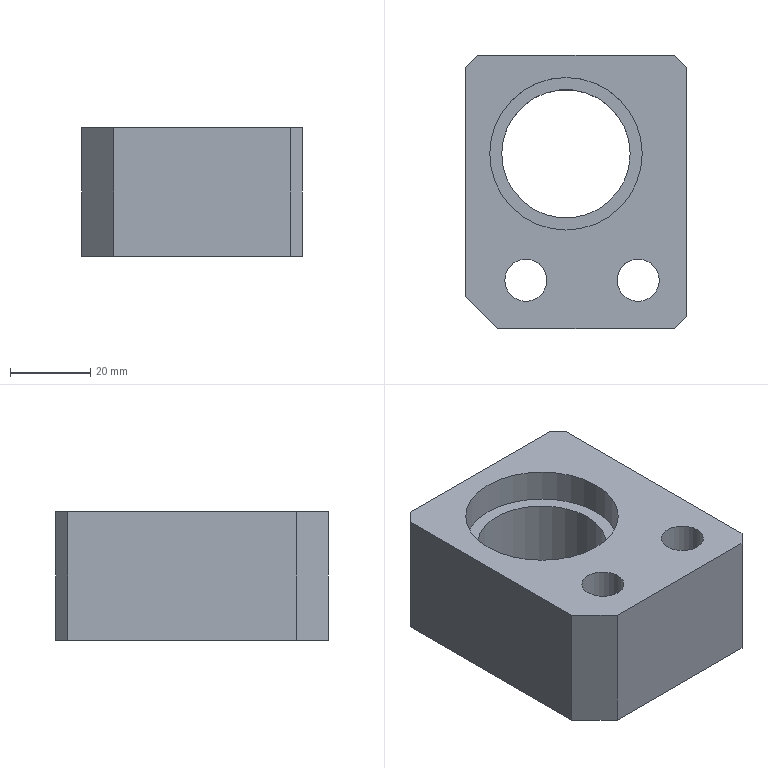Part | STEP file | lll_id3658_x_t | 1 solid | 19 faces | box 55 x 68 x 32 mm | volume 79468 mm3 | plane 13 | cylinder 6 | commonest cylinder face diameters 10.5 x2 17 x2 32 x1 38 x1
STEP:
#1=CARTESIAN_POINT('',(3324.617,172.788,77.5));
#2=VERTEX_POINT('',#1);
#3=CARTESIAN_POINT('',(3329.867,172.788,77.5));
#4=DIRECTION('',(0.,0.,1.));
#5=DIRECTION('',(-1.,0.,0.));
#6=AXIS2_PLACEMENT_3D('',#3,#4,#5);
#7=CIRCLE('',#6,5.25);
#8=EDGE_CURVE('',#2,#2,#7,.T.);
#9=ORIENTED_EDGE('',*,*,#8,.T.);
#10=EDGE_LOOP('',(#9));
#11=FACE_BOUND('',#10,.T.);
#12=CARTESIAN_POINT('',(3321.367,172.788,77.5));
#13=VERTEX_POINT('',#12);
#14=CARTESIAN_POINT('',(3329.867,172.788,77.5));
#15=DIRECTION('',(0.,0.,1.));
#16=DIRECTION('',(-1.,0.,0.));
#17=AXIS2_PLACEMENT_3D('',#14,#15,#16);
#18=CIRCLE('',#17,8.5);
#19=EDGE_CURVE('',#13,#13,#18,.T.);
#20=ORIENTED_EDGE('',*,*,#19,.F.);
#21=EDGE_LOOP('',(#20));
#22=FACE_BOUND('',#21,.T.);
#23=CARTESIAN_POINT('',(3329.867,172.788,77.5));
#24=DIRECTION('',(0.,0.,1.));
#25=DIRECTION('',(1.,0.,0.));
#26=AXIS2_PLACEMENT_3D('',#23,#24,#25);
#27=PLANE('',#26);
#28=ADVANCED_FACE('',(#11,#22),#27,.F.);
#29=CARTESIAN_POINT('',(3358.867,204.288,84.3));
#30=VERTEX_POINT('',#29);
#31=CARTESIAN_POINT('',(3339.867,204.288,84.3));
#32=DIRECTION('',(0.,0.,1.));
#33=DIRECTION('',(1.,0.,0.));
#34=AXIS2_PLACEMENT_3D('',#31,#32,#33);
#35=CIRCLE('',#34,19.);
#36=EDGE_CURVE('',#30,#30,#35,.T.);
#37=ORIENTED_EDGE('',*,*,#36,.T.);
#38=EDGE_LOOP('',(#37));
#39=FACE_BOUND('',#38,.T.);
#40=CARTESIAN_POINT('',(3355.867,204.288,84.3));
#41=VERTEX_POINT('',#40);
#42=CARTESIAN_POINT('',(3339.867,204.288,84.3));
#43=DIRECTION('',(0.,0.,1.));
#44=DIRECTION('',(1.,0.,0.));
#45=AXIS2_PLACEMENT_3D('',#42,#43,#44);
#46=CIRCLE('',#45,16.);
#47=EDGE_CURVE('',#41,#41,#46,.T.);
#48=ORIENTED_EDGE('',*,*,#47,.F.);
#49=EDGE_LOOP('',(#48));
#50=FACE_BOUND('',#49,.T.);
#51=CARTESIAN_POINT('',(3339.867,195.538,84.3));
#52=DIRECTION('',(0.,0.,-1.));
#53=DIRECTION('',(0.,-1.,0.));
#54=AXIS2_PLACEMENT_3D('',#51,#52,#53);
#55=PLANE('',#54);
#56=ADVANCED_FACE('',(#39,#50),#55,.F.);
#57=ORIENTED_EDGE('',*,*,#19,.T.);
#58=EDGE_LOOP('',(#57));
#59=FACE_BOUND('',#58,.T.);
#60=CARTESIAN_POINT('',(3321.367,172.788,60.5));
#61=VERTEX_POINT('',#60);
#62=CARTESIAN_POINT('',(3329.867,172.788,60.5));
#63=DIRECTION('',(0.,0.,-1.));
#64=DIRECTION('',(-1.,0.,0.));
#65=AXIS2_PLACEMENT_3D('',#62,#63,#64);
#66=CIRCLE('',#65,8.5);
#67=EDGE_CURVE('',#61,#61,#66,.T.);
#68=ORIENTED_EDGE('',*,*,#67,.T.);
#69=EDGE_LOOP('',(#68));
#70=FACE_BOUND('',#69,.T.);
#71=CARTESIAN_POINT('',(3329.867,172.788,60.5));
#72=DIRECTION('',(0.,0.,1.));
#73=DIRECTION('',(1.,0.,0.));
#74=AXIS2_PLACEMENT_3D('',#71,#72,#73);
#75=CYLINDRICAL_SURFACE('',#74,8.5);
#76=ADVANCED_FACE('',(#59,#70),#75,.F.);
#77=CARTESIAN_POINT('',(3314.867,225.788,60.5));
#78=VERTEX_POINT('',#77);
#79=CARTESIAN_POINT('',(3317.867,228.788,60.5));
#80=VERTEX_POINT('',#79);
#81=CARTESIAN_POINT('',(3334.05,244.97,60.5));
#82=DIRECTION('',(0.7071,0.7071,0.));
#83=VECTOR('',#82,1.);
#84=LINE('',#81,#83);
#85=EDGE_CURVE('',#78,#80,#84,.T.);
#86=ORIENTED_EDGE('',*,*,#85,.F.);
#87=CARTESIAN_POINT('',(3314.867,225.788,92.5));
#88=VERTEX_POINT('',#87);
#89=CARTESIAN_POINT('',(3314.867,225.788,-8.5));
#90=DIRECTION('',(0.,0.,-1.));
#91=VECTOR('',#90,1.);
#92=LINE('',#89,#91);
#93=EDGE_CURVE('',#88,#78,#92,.T.);
#94=ORIENTED_EDGE('',*,*,#93,.F.);
#95=CARTESIAN_POINT('',(3317.867,228.788,92.5));
#96=VERTEX_POINT('',#95);
#97=CARTESIAN_POINT('',(3334.05,244.97,92.5));
#98=DIRECTION('',(-0.7071,-0.7071,0.));
#99=VECTOR('',#98,1.);
#100=LINE('',#97,#99);
#101=EDGE_CURVE('',#96,#88,#100,.T.);
#102=ORIENTED_EDGE('',*,*,#101,.F.);
#103=CARTESIAN_POINT('',(3317.867,228.788,-8.5));
#104=DIRECTION('',(0.,0.,1.));
#105=VECTOR('',#104,1.);
#106=LINE('',#103,#105);
#107=EDGE_CURVE('',#80,#96,#106,.T.);
#108=ORIENTED_EDGE('',*,*,#107,.F.);
#109=EDGE_LOOP('',(#86,#94,#102,#108));
#110=FACE_OUTER_BOUND('',#109,.T.);
#111=CARTESIAN_POINT('',(3317.867,228.788,-8.5));
#112=DIRECTION('',(0.7071,-0.7071,0.));
#113=DIRECTION('',(0.,0.,1.));
#114=AXIS2_PLACEMENT_3D('',#111,#112,#113);
#115=PLANE('',#114);
#116=ADVANCED_FACE('',(#110),#115,.F.);
#117=CARTESIAN_POINT('',(3366.867,228.788,60.5));
#118=VERTEX_POINT('',#117);
#119=CARTESIAN_POINT('',(3403.057,228.788,60.5));
#120=DIRECTION('',(1.,0.,0.));
#121=VECTOR('',#120,1.);
#122=LINE('',#119,#121);
#123=EDGE_CURVE('',#80,#118,#122,.T.);
#124=ORIENTED_EDGE('',*,*,#123,.F.);
#125=ORIENTED_EDGE('',*,*,#107,.T.);
#126=CARTESIAN_POINT('',(3366.867,228.788,92.5));
#127=VERTEX_POINT('',#126);
#128=CARTESIAN_POINT('',(3339.867,228.788,92.5));
#129=DIRECTION('',(-1.,0.,0.));
#130=VECTOR('',#129,1.);
#131=LINE('',#128,#130);
#132=EDGE_CURVE('',#127,#96,#131,.T.);
#133=ORIENTED_EDGE('',*,*,#132,.F.);
#134=CARTESIAN_POINT('',(3366.867,228.788,-8.5));
#135=DIRECTION('',(0.,0.,1.));
#136=VECTOR('',#135,1.);
#137=LINE('',#134,#136);
#138=EDGE_CURVE('',#118,#127,#137,.T.);
#139=ORIENTED_EDGE('',*,*,#138,.F.);
#140=EDGE_LOOP('',(#124,#125,#133,#139));
#141=FACE_OUTER_BOUND('',#140,.T.);
#142=CARTESIAN_POINT('',(3339.867,228.788,-8.5));
#143=DIRECTION('',(0.,1.,0.));
#144=DIRECTION('',(0.,0.,-1.));
#145=AXIS2_PLACEMENT_3D('',#142,#143,#144);
#146=PLANE('',#145);
#147=ADVANCED_FACE('',(#141),#146,.T.);
#148=CARTESIAN_POINT('',(3369.867,225.788,92.5));
#149=VERTEX_POINT('',#148);
#150=CARTESIAN_POINT('',(3369.867,225.788,92.5));
#151=DIRECTION('',(0.7071,-0.7071,0.));
#152=VECTOR('',#151,1.);
#153=LINE('',#150,#152);
#154=EDGE_CURVE('',#127,#149,#153,.T.);
#155=ORIENTED_EDGE('',*,*,#154,.T.);
#156=CARTESIAN_POINT('',(3369.867,225.788,60.5));
#157=VERTEX_POINT('',#156);
#158=CARTESIAN_POINT('',(3369.867,225.788,-8.5));
#159=DIRECTION('',(0.,0.,-1.));
#160=VECTOR('',#159,1.);
#161=LINE('',#158,#160);
#162=EDGE_CURVE('',#149,#157,#161,.T.);
#163=ORIENTED_EDGE('',*,*,#162,.T.);
#164=CARTESIAN_POINT('',(3364.917,230.738,60.5));
#165=DIRECTION('',(-0.7071,0.7071,0.));
#166=VECTOR('',#165,1.);
#167=LINE('',#164,#166);
#168=EDGE_CURVE('',#157,#118,#167,.T.);
#169=ORIENTED_EDGE('',*,*,#168,.T.);
#170=ORIENTED_EDGE('',*,*,#138,.T.);
#171=EDGE_LOOP('',(#155,#163,#169,#170));
#172=FACE_OUTER_BOUND('',#171,.T.);
#173=CARTESIAN_POINT('',(3369.867,225.788,-8.5));
#174=DIRECTION('',(-0.7071,-0.7071,0.));
#175=DIRECTION('',(0.7071,-0.7071,0.));
#176=AXIS2_PLACEMENT_3D('',#173,#174,#175);
#177=PLANE('',#176);
#178=ADVANCED_FACE('',(#172),#177,.F.);
#179=CARTESIAN_POINT('',(3369.867,163.788,60.5));
#180=VERTEX_POINT('',#179);
#181=CARTESIAN_POINT('',(3369.867,178.012,60.5));
#182=DIRECTION('',(0.,-1.,0.));
#183=VECTOR('',#182,1.);
#184=LINE('',#181,#183);
#185=EDGE_CURVE('',#157,#180,#184,.T.);
#186=ORIENTED_EDGE('',*,*,#185,.F.);
#187=ORIENTED_EDGE('',*,*,#162,.F.);
#188=CARTESIAN_POINT('',(3369.867,163.788,92.5));
#189=VERTEX_POINT('',#188);
#190=CARTESIAN_POINT('',(3369.867,173.063,92.5));
#191=DIRECTION('',(0.,1.,0.));
#192=VECTOR('',#191,1.);
#193=LINE('',#190,#192);
#194=EDGE_CURVE('',#189,#149,#193,.T.);
#195=ORIENTED_EDGE('',*,*,#194,.F.);
#196=CARTESIAN_POINT('',(3369.867,163.788,-8.5));
#197=DIRECTION('',(0.,0.,1.));
#198=VECTOR('',#197,1.);
#199=LINE('',#196,#198);
#200=EDGE_CURVE('',#180,#189,#199,.T.);
#201=ORIENTED_EDGE('',*,*,#200,.F.);
#202=EDGE_LOOP('',(#186,#187,#195,#201));
#203=FACE_OUTER_BOUND('',#202,.T.);
#204=CARTESIAN_POINT('',(3369.867,204.288,-8.5));
#205=DIRECTION('',(1.,0.,0.));
#206=DIRECTION('',(0.,0.,-1.));
#207=AXIS2_PLACEMENT_3D('',#204,#205,#206);
#208=PLANE('',#207);
#209=ADVANCED_FACE('',(#203),#208,.T.);
#210=CARTESIAN_POINT('',(3366.867,160.788,92.5));
#211=VERTEX_POINT('',#210);
#212=CARTESIAN_POINT('',(3366.867,160.788,92.5));
#213=DIRECTION('',(-0.7071,-0.7071,0.));
#214=VECTOR('',#213,1.);
#215=LINE('',#212,#214);
#216=EDGE_CURVE('',#189,#211,#215,.T.);
#217=ORIENTED_EDGE('',*,*,#216,.T.);
#218=CARTESIAN_POINT('',(3366.867,160.788,60.5));
#219=VERTEX_POINT('',#218);
#220=CARTESIAN_POINT('',(3366.867,160.788,-8.5));
#221=DIRECTION('',(0.,0.,-1.));
#222=VECTOR('',#221,1.);
#223=LINE('',#220,#222);
#224=EDGE_CURVE('',#211,#219,#223,.T.);
#225=ORIENTED_EDGE('',*,*,#224,.T.);
#226=CARTESIAN_POINT('',(3366.867,160.788,60.5));
#227=DIRECTION('',(0.7071,0.7071,0.));
#228=VECTOR('',#227,1.);
#229=LINE('',#226,#228);
#230=EDGE_CURVE('',#219,#180,#229,.T.);
#231=ORIENTED_EDGE('',*,*,#230,.T.);
#232=ORIENTED_EDGE('',*,*,#200,.T.);
#233=EDGE_LOOP('',(#217,#225,#231,#232));
#234=FACE_OUTER_BOUND('',#233,.T.);
#235=CARTESIAN_POINT('',(3366.867,160.788,-8.5));
#236=DIRECTION('',(-0.7071,0.7071,0.));
#237=DIRECTION('',(-0.7071,-0.7071,0.));
#238=AXIS2_PLACEMENT_3D('',#235,#236,#237);
#239=PLANE('',#238);
#240=ADVANCED_FACE('',(#234),#239,.F.);
#241=CARTESIAN_POINT('',(3322.867,160.788,92.5));
#242=VERTEX_POINT('',#241);
#243=CARTESIAN_POINT('',(3339.867,160.788,92.5));
#244=DIRECTION('',(1.,0.,0.));
#245=VECTOR('',#244,1.);
#246=LINE('',#243,#245);
#247=EDGE_CURVE('',#242,#211,#246,.T.);
#248=ORIENTED_EDGE('',*,*,#247,.F.);
#249=CARTESIAN_POINT('',(3322.867,160.788,60.5));
#250=VERTEX_POINT('',#249);
#251=CARTESIAN_POINT('',(3322.867,160.788,-8.5));
#252=DIRECTION('',(0.,0.,-1.));
#253=VECTOR('',#252,1.);
#254=LINE('',#251,#253);
#255=EDGE_CURVE('',#242,#250,#254,.T.);
#256=ORIENTED_EDGE('',*,*,#255,.T.);
#257=CARTESIAN_POINT('',(3403.057,160.788,60.5));
#258=DIRECTION('',(-1.,0.,0.));
#259=VECTOR('',#258,1.);
#260=LINE('',#257,#259);
#261=EDGE_CURVE('',#219,#250,#260,.T.);
#262=ORIENTED_EDGE('',*,*,#261,.F.);
#263=ORIENTED_EDGE('',*,*,#224,.F.);
#264=EDGE_LOOP('',(#248,#256,#262,#263));
#265=FACE_OUTER_BOUND('',#264,.T.);
#266=CARTESIAN_POINT('',(3339.867,160.788,-8.5));
#267=DIRECTION('',(0.,-1.,0.));
#268=DIRECTION('',(0.,0.,1.));
#269=AXIS2_PLACEMENT_3D('',#266,#267,#268);
#270=PLANE('',#269);
#271=ADVANCED_FACE('',(#265),#270,.T.);
#272=CARTESIAN_POINT('',(3314.867,168.788,92.5));
#273=VERTEX_POINT('',#272);
#274=CARTESIAN_POINT('',(3358.275,125.381,92.5));
#275=DIRECTION('',(0.7071,-0.7071,0.));
#276=VECTOR('',#275,1.);
#277=LINE('',#274,#276);
#278=EDGE_CURVE('',#273,#242,#277,.T.);
#279=ORIENTED_EDGE('',*,*,#278,.F.);
#280=CARTESIAN_POINT('',(3314.867,168.788,60.5));
#281=VERTEX_POINT('',#280);
#282=CARTESIAN_POINT('',(3314.867,168.788,-8.5));
#283=DIRECTION('',(0.,0.,1.));
#284=VECTOR('',#283,1.);
#285=LINE('',#282,#284);
#286=EDGE_CURVE('',#281,#273,#285,.T.);
#287=ORIENTED_EDGE('',*,*,#286,.F.);
#288=CARTESIAN_POINT('',(3353.325,130.33,60.5));
#289=DIRECTION('',(-0.7071,0.7071,0.));
#290=VECTOR('',#289,1.);
#291=LINE('',#288,#290);
#292=EDGE_CURVE('',#250,#281,#291,.T.);
#293=ORIENTED_EDGE('',*,*,#292,.F.);
#294=ORIENTED_EDGE('',*,*,#255,.F.);
#295=EDGE_LOOP('',(#279,#287,#293,#294));
#296=FACE_OUTER_BOUND('',#295,.T.);
#297=CARTESIAN_POINT('',(3322.867,160.788,-8.5));
#298=DIRECTION('',(0.7071,0.7071,0.));
#299=DIRECTION('',(0.,0.,-1.));
#300=AXIS2_PLACEMENT_3D('',#297,#298,#299);
#301=PLANE('',#300);
#302=ADVANCED_FACE('',(#296),#301,.F.);
#303=CARTESIAN_POINT('',(3314.867,178.012,60.5));
#304=DIRECTION('',(0.,1.,0.));
#305=VECTOR('',#304,1.);
#306=LINE('',#303,#305);
#307=EDGE_CURVE('',#281,#78,#306,.T.);
#308=ORIENTED_EDGE('',*,*,#307,.F.);
#309=ORIENTED_EDGE('',*,*,#286,.T.);
#310=CARTESIAN_POINT('',(3314.867,178.012,92.5));
#311=DIRECTION('',(0.,-1.,0.));
#312=VECTOR('',#311,1.);
#313=LINE('',#310,#312);
#314=EDGE_CURVE('',#88,#273,#313,.T.);
#315=ORIENTED_EDGE('',*,*,#314,.F.);
#316=ORIENTED_EDGE('',*,*,#93,.T.);
#317=EDGE_LOOP('',(#308,#309,#315,#316));
#318=FACE_OUTER_BOUND('',#317,.T.);
#319=CARTESIAN_POINT('',(3314.867,209.238,-8.5));
#320=DIRECTION('',(-1.,0.,0.));
#321=DIRECTION('',(0.,0.,1.));
#322=AXIS2_PLACEMENT_3D('',#319,#320,#321);
#323=PLANE('',#322);
#324=ADVANCED_FACE('',(#318),#323,.T.);
#325=CARTESIAN_POINT('',(3324.617,172.788,92.5));
#326=VERTEX_POINT('',#325);
#327=CARTESIAN_POINT('',(3329.867,172.788,92.5));
#328=DIRECTION('',(0.,0.,-1.));
#329=DIRECTION('',(-1.,0.,0.));
#330=AXIS2_PLACEMENT_3D('',#327,#328,#329);
#331=CIRCLE('',#330,5.25);
#332=EDGE_CURVE('',#326,#326,#331,.T.);
#333=ORIENTED_EDGE('',*,*,#332,.F.);
#334=EDGE_LOOP('',(#333));
#335=FACE_BOUND('',#334,.T.);
#336=ORIENTED_EDGE('',*,*,#8,.F.);
#337=EDGE_LOOP('',(#336));
#338=FACE_BOUND('',#337,.T.);
#339=CARTESIAN_POINT('',(3329.867,172.788,160.5));
#340=DIRECTION('',(0.,0.,1.));
#341=DIRECTION('',(1.,0.,0.));
#342=AXIS2_PLACEMENT_3D('',#339,#340,#341);
#343=CYLINDRICAL_SURFACE('',#342,5.25);
#344=ADVANCED_FACE('',(#335,#338),#343,.F.);
#345=CARTESIAN_POINT('',(3320.867,204.288,92.5));
#346=VERTEX_POINT('',#345);
#347=CARTESIAN_POINT('',(3339.867,204.288,92.5));
#348=DIRECTION('',(0.,0.,-1.));
#349=DIRECTION('',(-1.,0.,0.));
#350=AXIS2_PLACEMENT_3D('',#347,#348,#349);
#351=CIRCLE('',#350,19.);
#352=EDGE_CURVE('',#346,#346,#351,.T.);
#353=ORIENTED_EDGE('',*,*,#352,.F.);
#354=EDGE_LOOP('',(#353));
#355=FACE_BOUND('',#354,.T.);
#356=ORIENTED_EDGE('',*,*,#36,.F.);
#357=EDGE_LOOP('',(#356));
#358=FACE_BOUND('',#357,.T.);
#359=CARTESIAN_POINT('',(3339.867,204.288,90.));
#360=DIRECTION('',(0.,0.,-1.));
#361=DIRECTION('',(0.,1.,0.));
#362=AXIS2_PLACEMENT_3D('',#359,#360,#361);
#363=CYLINDRICAL_SURFACE('',#362,19.);
#364=ADVANCED_FACE('',(#355,#358),#363,.F.);
#365=CARTESIAN_POINT('',(3363.117,172.788,92.5));
#366=VERTEX_POINT('',#365);
#367=CARTESIAN_POINT('',(3357.867,172.788,92.5));
#368=DIRECTION('',(0.,0.,1.));
#369=DIRECTION('',(1.,0.,0.));
#370=AXIS2_PLACEMENT_3D('',#367,#368,#369);
#371=CIRCLE('',#370,5.25);
#372=EDGE_CURVE('',#366,#366,#371,.T.);
#373=ORIENTED_EDGE('',*,*,#372,.F.);
#374=EDGE_LOOP('',(#373));
#375=FACE_BOUND('',#374,.T.);
#376=ORIENTED_EDGE('',*,*,#352,.T.);
#377=EDGE_LOOP('',(#376));
#378=FACE_BOUND('',#377,.T.);
#379=ORIENTED_EDGE('',*,*,#332,.T.);
#380=EDGE_LOOP('',(#379));
#381=FACE_BOUND('',#380,.T.);
#382=ORIENTED_EDGE('',*,*,#314,.T.);
#383=ORIENTED_EDGE('',*,*,#278,.T.);
#384=ORIENTED_EDGE('',*,*,#247,.T.);
#385=ORIENTED_EDGE('',*,*,#216,.F.);
#386=ORIENTED_EDGE('',*,*,#194,.T.);
#387=ORIENTED_EDGE('',*,*,#154,.F.);
#388=ORIENTED_EDGE('',*,*,#132,.T.);
#389=ORIENTED_EDGE('',*,*,#101,.T.);
#390=EDGE_LOOP('',(#382,#383,#384,#385,#386,#387,#388,#389));
#391=FACE_BOUND('',#390,.T.);
#392=CARTESIAN_POINT('',(3408.007,173.063,92.5));
#393=DIRECTION('',(0.,0.,1.));
#394=DIRECTION('',(1.,0.,0.));
#395=AXIS2_PLACEMENT_3D('',#392,#393,#394);
#396=PLANE('',#395);
#397=ADVANCED_FACE('',(#375,#378,#381,#391),#396,.T.);
#398=CARTESIAN_POINT('',(3323.867,204.288,60.5));
#399=VERTEX_POINT('',#398);
#400=CARTESIAN_POINT('',(3339.867,204.288,60.5));
#401=DIRECTION('',(0.,0.,1.));
#402=DIRECTION('',(-1.,0.,0.));
#403=AXIS2_PLACEMENT_3D('',#400,#401,#402);
#404=CIRCLE('',#403,16.);
#405=EDGE_CURVE('',#399,#399,#404,.T.);
#406=ORIENTED_EDGE('',*,*,#405,.F.);
#407=EDGE_LOOP('',(#406));
#408=FACE_BOUND('',#407,.T.);
#409=ORIENTED_EDGE('',*,*,#47,.T.);
#410=EDGE_LOOP('',(#409));
#411=FACE_BOUND('',#410,.T.);
#412=CARTESIAN_POINT('',(3339.867,204.288,44.8));
#413=DIRECTION('',(0.,0.,-1.));
#414=DIRECTION('',(0.,1.,0.));
#415=AXIS2_PLACEMENT_3D('',#412,#413,#414);
#416=CYLINDRICAL_SURFACE('',#415,16.);
#417=ADVANCED_FACE('',(#408,#411),#416,.F.);
#418=CARTESIAN_POINT('',(3366.367,172.788,60.5));
#419=VERTEX_POINT('',#418);
#420=CARTESIAN_POINT('',(3357.867,172.788,60.5));
#421=DIRECTION('',(0.,0.,-1.));
#422=DIRECTION('',(1.,0.,0.));
#423=AXIS2_PLACEMENT_3D('',#420,#421,#422);
#424=CIRCLE('',#423,8.5);
#425=EDGE_CURVE('',#419,#419,#424,.T.);
#426=ORIENTED_EDGE('',*,*,#425,.F.);
#427=EDGE_LOOP('',(#426));
#428=FACE_BOUND('',#427,.T.);
#429=ORIENTED_EDGE('',*,*,#405,.T.);
#430=EDGE_LOOP('',(#429));
#431=FACE_BOUND('',#430,.T.);
#432=ORIENTED_EDGE('',*,*,#261,.T.);
#433=ORIENTED_EDGE('',*,*,#292,.T.);
#434=ORIENTED_EDGE('',*,*,#307,.T.);
#435=ORIENTED_EDGE('',*,*,#85,.T.);
#436=ORIENTED_EDGE('',*,*,#123,.T.);
#437=ORIENTED_EDGE('',*,*,#168,.F.);
#438=ORIENTED_EDGE('',*,*,#185,.T.);
#439=ORIENTED_EDGE('',*,*,#230,.F.);
#440=EDGE_LOOP('',(#432,#433,#434,#435,#436,#437,#438,#439));
#441=FACE_BOUND('',#440,.T.);
#442=ORIENTED_EDGE('',*,*,#67,.F.);
#443=EDGE_LOOP('',(#442));
#444=FACE_BOUND('',#443,.T.);
#445=CARTESIAN_POINT('',(3403.057,178.012,60.5));
#446=DIRECTION('',(0.,0.,1.));
#447=DIRECTION('',(1.,0.,0.));
#448=AXIS2_PLACEMENT_3D('',#445,#446,#447);
#449=PLANE('',#448);
#450=ADVANCED_FACE('',(#428,#431,#441,#444),#449,.F.);
#451=CARTESIAN_POINT('',(3352.617,172.788,77.5));
#452=VERTEX_POINT('',#451);
#453=CARTESIAN_POINT('',(3357.867,172.788,77.5));
#454=DIRECTION('',(0.,0.,1.));
#455=DIRECTION('',(-1.,0.,0.));
#456=AXIS2_PLACEMENT_3D('',#453,#454,#455);
#457=CIRCLE('',#456,5.25);
#458=EDGE_CURVE('',#452,#452,#457,.T.);
#459=ORIENTED_EDGE('',*,*,#458,.T.);
#460=EDGE_LOOP('',(#459));
#461=FACE_BOUND('',#460,.T.);
#462=CARTESIAN_POINT('',(3349.367,172.788,77.5));
#463=VERTEX_POINT('',#462);
#464=CARTESIAN_POINT('',(3357.867,172.788,77.5));
#465=DIRECTION('',(0.,0.,1.));
#466=DIRECTION('',(-1.,0.,0.));
#467=AXIS2_PLACEMENT_3D('',#464,#465,#466);
#468=CIRCLE('',#467,8.5);
#469=EDGE_CURVE('',#463,#463,#468,.T.);
#470=ORIENTED_EDGE('',*,*,#469,.F.);
#471=EDGE_LOOP('',(#470));
#472=FACE_BOUND('',#471,.T.);
#473=CARTESIAN_POINT('',(3357.867,172.788,77.5));
#474=DIRECTION('',(0.,0.,1.));
#475=DIRECTION('',(1.,0.,0.));
#476=AXIS2_PLACEMENT_3D('',#473,#474,#475);
#477=PLANE('',#476);
#478=ADVANCED_FACE('',(#461,#472),#477,.F.);
#479=ORIENTED_EDGE('',*,*,#372,.T.);
#480=EDGE_LOOP('',(#479));
#481=FACE_BOUND('',#480,.T.);
#482=ORIENTED_EDGE('',*,*,#458,.F.);
#483=EDGE_LOOP('',(#482));
#484=FACE_BOUND('',#483,.T.);
#485=CARTESIAN_POINT('',(3357.867,172.788,160.5));
#486=DIRECTION('',(0.,0.,1.));
#487=DIRECTION('',(1.,0.,0.));
#488=AXIS2_PLACEMENT_3D('',#485,#486,#487);
#489=CYLINDRICAL_SURFACE('',#488,5.25);
#490=ADVANCED_FACE('',(#481,#484),#489,.F.);
#491=ORIENTED_EDGE('',*,*,#469,.T.);
#492=EDGE_LOOP('',(#491));
#493=FACE_BOUND('',#492,.T.);
#494=ORIENTED_EDGE('',*,*,#425,.T.);
#495=EDGE_LOOP('',(#494));
#496=FACE_BOUND('',#495,.T.);
#497=CARTESIAN_POINT('',(3357.867,172.788,60.5));
#498=DIRECTION('',(0.,0.,1.));
#499=DIRECTION('',(1.,0.,0.));
#500=AXIS2_PLACEMENT_3D('',#497,#498,#499);
#501=CYLINDRICAL_SURFACE('',#500,8.5);
#502=ADVANCED_FACE('',(#493,#496),#501,.F.);
#503=CLOSED_SHELL('',(#28,#56,#76,#116,#147,#178,#209,#240,#271,#302,#324,#344,#364,#397,#417,#450,#478,#490,#502));
#504=MANIFOLD_SOLID_BREP('',#503);
#505=(LENGTH_UNIT()NAMED_UNIT(*)SI_UNIT(.MILLI.,.METRE.));
#506=UNCERTAINTY_MEASURE_WITH_UNIT(LENGTH_MEASURE(0.00002),#505,'','');
#507=(NAMED_UNIT(*)PLANE_ANGLE_UNIT()SI_UNIT($,.RADIAN.));
#508=PLANE_ANGLE_MEASURE_WITH_UNIT(PLANE_ANGLE_MEASURE(0.01745),#507);
#509=DIMENSIONAL_EXPONENTS(0.,0.,0.,0.,0.,0.,0.);
#510=(CONVERSION_BASED_UNIT('DEGREE',#508)NAMED_UNIT(#509)PLANE_ANGLE_UNIT());
#511=(NAMED_UNIT(*)SI_UNIT($,.STERADIAN.)SOLID_ANGLE_UNIT());
#512=(GEOMETRIC_REPRESENTATION_CONTEXT(3)GLOBAL_UNCERTAINTY_ASSIGNED_CONTEXT((#506))GLOBAL_UNIT_ASSIGNED_CONTEXT((#505,#510,#511))REPRESENTATION_CONTEXT('',''));
#513=ADVANCED_BREP_SHAPE_REPRESENTATION('',(#504),#512);